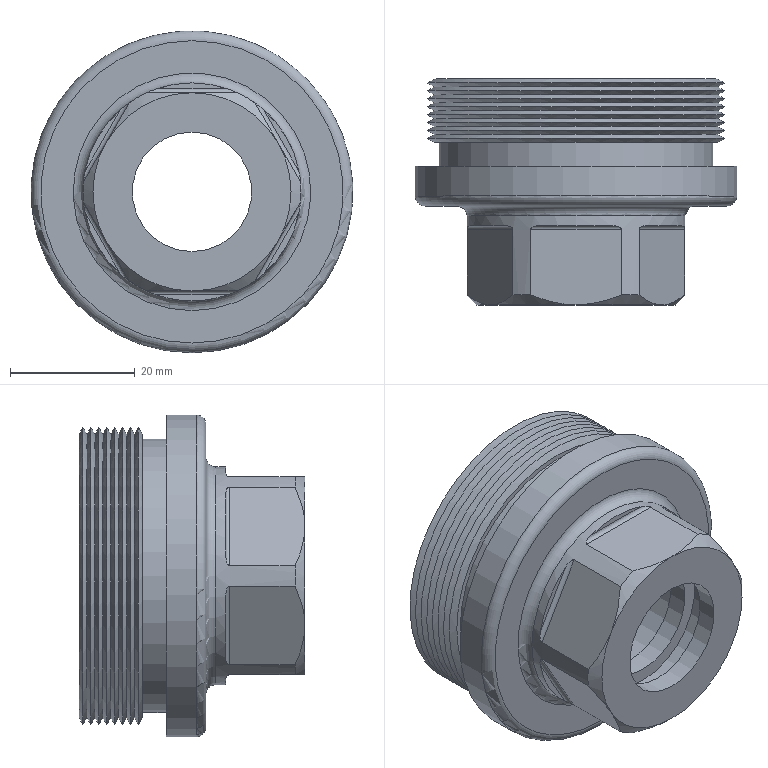Part | NX | features MG0330 trunion parts 24(trunion group) 2 | 1 solid | 63 faces | box 51.598 x 36.22 x 51.598 mm | volume 23694 mm3 | plane 23 | cone 22 | cylinder 16 | torus 2 | commonest cylinder face diameters 1.27 x6 19.152 x2 38.1 x2 22.228 x1 23.444 x1 34.925 x1